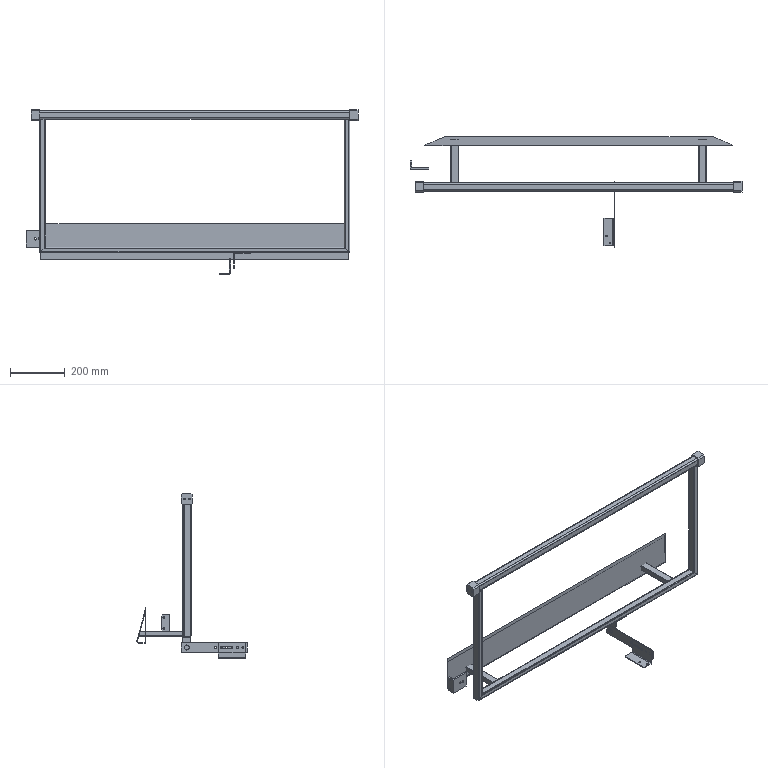Part | SolidWorks | 11 solids | 257 faces | box 1215 x 402.556 x 603 mm | volume 1534055 mm3 | plane 148 | cylinder 105 | cone 4 | commonest cylinder face diameters 4 x14 6.5 x14 8 x13 6 x12 7 x12 2 x8